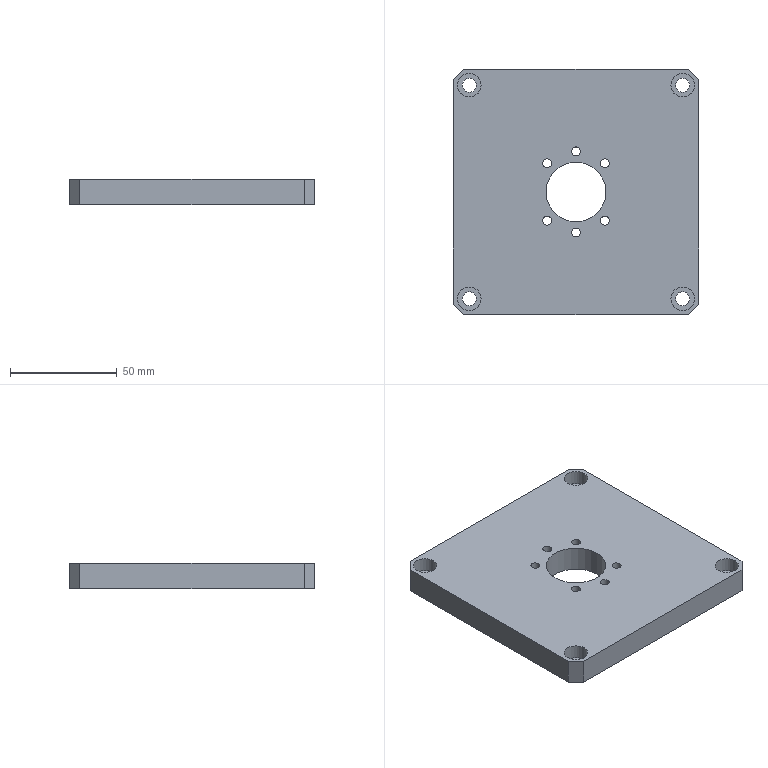Part | NX | 1 solid | 33 faces | box 115 x 115 x 12 mm | volume 146316 mm3 | cylinder 17 | plane 14 | cone 2 | commonest cylinder face diameters 4.2 x6 6.6 x4 11 x4 2.5 x2 28 x1
STEP:
#1=CARTESIAN_POINT('',(52.5,-57.5,6.));
#2=VERTEX_POINT('',#1);
#3=CARTESIAN_POINT('',(57.5,-52.5,6.));
#4=VERTEX_POINT('',#3);
#5=CARTESIAN_POINT('',(55.,-55.,6.));
#6=DIRECTION('',(0.7071,0.7071,0.));
#7=VECTOR('',#6,1000.);
#8=LINE('',#5,#7);
#9=EDGE_CURVE('',#2,#4,#8,.T.);
#10=ORIENTED_EDGE('',*,*,#9,.F.);
#11=CARTESIAN_POINT('',(52.5,-57.5,-6.));
#12=VERTEX_POINT('',#11);
#13=CARTESIAN_POINT('',(52.5,-57.5,6.));
#14=DIRECTION('',(0.,0.,1.));
#15=VECTOR('',#14,1000.);
#16=LINE('',#13,#15);
#17=EDGE_CURVE('',#12,#2,#16,.T.);
#18=ORIENTED_EDGE('',*,*,#17,.F.);
#19=CARTESIAN_POINT('',(57.5,-52.5,-6.));
#20=VERTEX_POINT('',#19);
#21=CARTESIAN_POINT('',(57.5,-52.5,-6.));
#22=DIRECTION('',(-0.7071,-0.7071,0.));
#23=VECTOR('',#22,1000.);
#24=LINE('',#21,#23);
#25=EDGE_CURVE('',#20,#12,#24,.T.);
#26=ORIENTED_EDGE('',*,*,#25,.F.);
#27=CARTESIAN_POINT('',(57.5,-52.5,6.));
#28=DIRECTION('',(0.,0.,-1.));
#29=VECTOR('',#28,1000.);
#30=LINE('',#27,#29);
#31=EDGE_CURVE('',#4,#20,#30,.T.);
#32=ORIENTED_EDGE('',*,*,#31,.F.);
#33=EDGE_LOOP('',(#10,#18,#26,#32));
#34=FACE_BOUND('',#33,.T.);
#35=CARTESIAN_POINT('',(57.5,-52.5,6.));
#36=DIRECTION('',(-0.7071,0.7071,0.));
#37=DIRECTION('',(0.,0.,-1.));
#38=AXIS2_PLACEMENT_3D('',#35,#36,#37);
#39=PLANE('',#38);
#40=ADVANCED_FACE('',(#34),#39,.F.);
#41=CARTESIAN_POINT('',(-57.5,-52.5,6.));
#42=VERTEX_POINT('',#41);
#43=CARTESIAN_POINT('',(-52.5,-57.5,6.));
#44=VERTEX_POINT('',#43);
#45=CARTESIAN_POINT('',(-55.,-55.,6.));
#46=DIRECTION('',(0.7071,-0.7071,0.));
#47=VECTOR('',#46,1000.);
#48=LINE('',#45,#47);
#49=EDGE_CURVE('',#42,#44,#48,.T.);
#50=ORIENTED_EDGE('',*,*,#49,.F.);
#51=CARTESIAN_POINT('',(-57.5,-52.5,-6.));
#52=VERTEX_POINT('',#51);
#53=CARTESIAN_POINT('',(-57.5,-52.5,6.));
#54=DIRECTION('',(0.,0.,1.));
#55=VECTOR('',#54,1000.);
#56=LINE('',#53,#55);
#57=EDGE_CURVE('',#52,#42,#56,.T.);
#58=ORIENTED_EDGE('',*,*,#57,.F.);
#59=CARTESIAN_POINT('',(-52.5,-57.5,-6.));
#60=VERTEX_POINT('',#59);
#61=CARTESIAN_POINT('',(-52.5,-57.5,-6.));
#62=DIRECTION('',(-0.7071,0.7071,0.));
#63=VECTOR('',#62,1000.);
#64=LINE('',#61,#63);
#65=EDGE_CURVE('',#60,#52,#64,.T.);
#66=ORIENTED_EDGE('',*,*,#65,.F.);
#67=CARTESIAN_POINT('',(-52.5,-57.5,6.));
#68=DIRECTION('',(0.,0.,-1.));
#69=VECTOR('',#68,1000.);
#70=LINE('',#67,#69);
#71=EDGE_CURVE('',#44,#60,#70,.T.);
#72=ORIENTED_EDGE('',*,*,#71,.F.);
#73=EDGE_LOOP('',(#50,#58,#66,#72));
#74=FACE_BOUND('',#73,.T.);
#75=CARTESIAN_POINT('',(-52.5,-57.5,6.));
#76=DIRECTION('',(0.7071,0.7071,0.));
#77=DIRECTION('',(0.,0.,-1.));
#78=AXIS2_PLACEMENT_3D('',#75,#76,#77);
#79=PLANE('',#78);
#80=ADVANCED_FACE('',(#74),#79,.F.);
#81=CARTESIAN_POINT('',(57.5,52.5,6.));
#82=VERTEX_POINT('',#81);
#83=CARTESIAN_POINT('',(52.5,57.5,6.));
#84=VERTEX_POINT('',#83);
#85=CARTESIAN_POINT('',(55.,55.,6.));
#86=DIRECTION('',(-0.7071,0.7071,0.));
#87=VECTOR('',#86,1000.);
#88=LINE('',#85,#87);
#89=EDGE_CURVE('',#82,#84,#88,.T.);
#90=ORIENTED_EDGE('',*,*,#89,.F.);
#91=CARTESIAN_POINT('',(57.5,52.5,-6.));
#92=VERTEX_POINT('',#91);
#93=CARTESIAN_POINT('',(57.5,52.5,6.));
#94=DIRECTION('',(0.,0.,1.));
#95=VECTOR('',#94,1000.);
#96=LINE('',#93,#95);
#97=EDGE_CURVE('',#92,#82,#96,.T.);
#98=ORIENTED_EDGE('',*,*,#97,.F.);
#99=CARTESIAN_POINT('',(52.5,57.5,-6.));
#100=VERTEX_POINT('',#99);
#101=CARTESIAN_POINT('',(52.5,57.5,-6.));
#102=DIRECTION('',(0.7071,-0.7071,0.));
#103=VECTOR('',#102,1000.);
#104=LINE('',#101,#103);
#105=EDGE_CURVE('',#100,#92,#104,.T.);
#106=ORIENTED_EDGE('',*,*,#105,.F.);
#107=CARTESIAN_POINT('',(52.5,57.5,6.));
#108=DIRECTION('',(0.,0.,-1.));
#109=VECTOR('',#108,1000.);
#110=LINE('',#107,#109);
#111=EDGE_CURVE('',#84,#100,#110,.T.);
#112=ORIENTED_EDGE('',*,*,#111,.F.);
#113=EDGE_LOOP('',(#90,#98,#106,#112));
#114=FACE_BOUND('',#113,.T.);
#115=CARTESIAN_POINT('',(52.5,57.5,6.));
#116=DIRECTION('',(-0.7071,-0.7071,0.));
#117=DIRECTION('',(0.,0.,-1.));
#118=AXIS2_PLACEMENT_3D('',#115,#116,#117);
#119=PLANE('',#118);
#120=ADVANCED_FACE('',(#114),#119,.F.);
#121=CARTESIAN_POINT('',(-52.5,57.5,6.));
#122=VERTEX_POINT('',#121);
#123=CARTESIAN_POINT('',(-57.5,52.5,6.));
#124=VERTEX_POINT('',#123);
#125=CARTESIAN_POINT('',(-55.,55.,6.));
#126=DIRECTION('',(-0.7071,-0.7071,0.));
#127=VECTOR('',#126,1000.);
#128=LINE('',#125,#127);
#129=EDGE_CURVE('',#122,#124,#128,.T.);
#130=ORIENTED_EDGE('',*,*,#129,.F.);
#131=CARTESIAN_POINT('',(-52.5,57.5,-6.));
#132=VERTEX_POINT('',#131);
#133=CARTESIAN_POINT('',(-52.5,57.5,6.));
#134=DIRECTION('',(0.,0.,1.));
#135=VECTOR('',#134,1000.);
#136=LINE('',#133,#135);
#137=EDGE_CURVE('',#132,#122,#136,.T.);
#138=ORIENTED_EDGE('',*,*,#137,.F.);
#139=CARTESIAN_POINT('',(-57.5,52.5,-6.));
#140=VERTEX_POINT('',#139);
#141=CARTESIAN_POINT('',(-57.5,52.5,-6.));
#142=DIRECTION('',(0.7071,0.7071,0.));
#143=VECTOR('',#142,1000.);
#144=LINE('',#141,#143);
#145=EDGE_CURVE('',#140,#132,#144,.T.);
#146=ORIENTED_EDGE('',*,*,#145,.F.);
#147=CARTESIAN_POINT('',(-57.5,52.5,6.));
#148=DIRECTION('',(0.,0.,-1.));
#149=VECTOR('',#148,1000.);
#150=LINE('',#147,#149);
#151=EDGE_CURVE('',#124,#140,#150,.T.);
#152=ORIENTED_EDGE('',*,*,#151,.F.);
#153=EDGE_LOOP('',(#130,#138,#146,#152));
#154=FACE_BOUND('',#153,.T.);
#155=CARTESIAN_POINT('',(-57.5,52.5,6.));
#156=DIRECTION('',(0.7071,-0.7071,0.));
#157=DIRECTION('',(0.,0.,-1.));
#158=AXIS2_PLACEMENT_3D('',#155,#156,#157);
#159=PLANE('',#158);
#160=ADVANCED_FACE('',(#154),#159,.F.);
#161=CARTESIAN_POINT('',(55.5,50.,-0.8));
#162=VERTEX_POINT('',#161);
#163=CARTESIAN_POINT('',(50.,50.,-0.8));
#164=DIRECTION('',(0.,0.,1.));
#165=DIRECTION('',(1.,0.,0.));
#166=AXIS2_PLACEMENT_3D('',#163,#164,#165);
#167=CIRCLE('',#166,5.5);
#168=EDGE_CURVE('',#162,#162,#167,.T.);
#169=ORIENTED_EDGE('',*,*,#168,.T.);
#170=EDGE_LOOP('',(#169));
#171=FACE_BOUND('',#170,.T.);
#172=CARTESIAN_POINT('',(53.3,50.,-0.8));
#173=VERTEX_POINT('',#172);
#174=CARTESIAN_POINT('',(50.,50.,-0.8));
#175=DIRECTION('',(0.,0.,1.));
#176=DIRECTION('',(1.,0.,0.));
#177=AXIS2_PLACEMENT_3D('',#174,#175,#176);
#178=CIRCLE('',#177,3.3);
#179=EDGE_CURVE('',#173,#173,#178,.T.);
#180=ORIENTED_EDGE('',*,*,#179,.F.);
#181=EDGE_LOOP('',(#180));
#182=FACE_BOUND('',#181,.T.);
#183=CARTESIAN_POINT('',(53.3,50.,-0.8));
#184=DIRECTION('',(0.,0.,-1.));
#185=DIRECTION('',(-1.,0.,0.));
#186=AXIS2_PLACEMENT_3D('',#183,#184,#185);
#187=PLANE('',#186);
#188=ADVANCED_FACE('',(#171,#182),#187,.F.);
#189=CARTESIAN_POINT('',(-55.5,50.,-0.8));
#190=VERTEX_POINT('',#189);
#191=CARTESIAN_POINT('',(-50.,50.,-0.8));
#192=DIRECTION('',(0.,0.,1.));
#193=DIRECTION('',(-1.,0.,0.));
#194=AXIS2_PLACEMENT_3D('',#191,#192,#193);
#195=CIRCLE('',#194,5.5);
#196=EDGE_CURVE('',#190,#190,#195,.T.);
#197=ORIENTED_EDGE('',*,*,#196,.T.);
#198=EDGE_LOOP('',(#197));
#199=FACE_BOUND('',#198,.T.);
#200=CARTESIAN_POINT('',(-53.3,50.,-0.8));
#201=VERTEX_POINT('',#200);
#202=CARTESIAN_POINT('',(-50.,50.,-0.8));
#203=DIRECTION('',(0.,0.,1.));
#204=DIRECTION('',(-1.,0.,0.));
#205=AXIS2_PLACEMENT_3D('',#202,#203,#204);
#206=CIRCLE('',#205,3.3);
#207=EDGE_CURVE('',#201,#201,#206,.T.);
#208=ORIENTED_EDGE('',*,*,#207,.F.);
#209=EDGE_LOOP('',(#208));
#210=FACE_BOUND('',#209,.T.);
#211=CARTESIAN_POINT('',(53.3,50.,-0.8));
#212=DIRECTION('',(0.,0.,-1.));
#213=DIRECTION('',(-1.,0.,0.));
#214=AXIS2_PLACEMENT_3D('',#211,#212,#213);
#215=PLANE('',#214);
#216=ADVANCED_FACE('',(#199,#210),#215,.F.);
#217=CARTESIAN_POINT('',(53.3,-50.,-6.));
#218=VERTEX_POINT('',#217);
#219=CARTESIAN_POINT('',(50.,-50.,-6.));
#220=DIRECTION('',(0.,0.,1.));
#221=DIRECTION('',(1.,0.,0.));
#222=AXIS2_PLACEMENT_3D('',#219,#220,#221);
#223=CIRCLE('',#222,3.3);
#224=EDGE_CURVE('',#218,#218,#223,.T.);
#225=ORIENTED_EDGE('',*,*,#224,.T.);
#226=EDGE_LOOP('',(#225));
#227=FACE_BOUND('',#226,.T.);
#228=CARTESIAN_POINT('',(-46.7,-50.,-6.));
#229=VERTEX_POINT('',#228);
#230=CARTESIAN_POINT('',(-50.,-50.,-6.));
#231=DIRECTION('',(0.,0.,1.));
#232=DIRECTION('',(1.,0.,0.));
#233=AXIS2_PLACEMENT_3D('',#230,#231,#232);
#234=CIRCLE('',#233,3.3);
#235=EDGE_CURVE('',#229,#229,#234,.T.);
#236=ORIENTED_EDGE('',*,*,#235,.T.);
#237=EDGE_LOOP('',(#236));
#238=FACE_BOUND('',#237,.T.);
#239=CARTESIAN_POINT('',(-57.5,57.5,-6.));
#240=DIRECTION('',(0.,-1.,0.));
#241=VECTOR('',#240,1000.);
#242=LINE('',#239,#241);
#243=EDGE_CURVE('',#140,#52,#242,.T.);
#244=ORIENTED_EDGE('',*,*,#243,.F.);
#245=ORIENTED_EDGE('',*,*,#145,.T.);
#246=CARTESIAN_POINT('',(-57.5,57.5,-6.));
#247=DIRECTION('',(-1.,0.,0.));
#248=VECTOR('',#247,1000.);
#249=LINE('',#246,#248);
#250=EDGE_CURVE('',#100,#132,#249,.T.);
#251=ORIENTED_EDGE('',*,*,#250,.F.);
#252=ORIENTED_EDGE('',*,*,#105,.T.);
#253=CARTESIAN_POINT('',(57.5,57.5,-6.));
#254=DIRECTION('',(0.,1.,0.));
#255=VECTOR('',#254,1000.);
#256=LINE('',#253,#255);
#257=EDGE_CURVE('',#20,#92,#256,.T.);
#258=ORIENTED_EDGE('',*,*,#257,.F.);
#259=ORIENTED_EDGE('',*,*,#25,.T.);
#260=CARTESIAN_POINT('',(-57.5,-57.5,-6.));
#261=DIRECTION('',(1.,0.,0.));
#262=VECTOR('',#261,1000.);
#263=LINE('',#260,#262);
#264=EDGE_CURVE('',#60,#12,#263,.T.);
#265=ORIENTED_EDGE('',*,*,#264,.F.);
#266=ORIENTED_EDGE('',*,*,#65,.T.);
#267=EDGE_LOOP('',(#244,#245,#251,#252,#258,#259,#265,#266));
#268=FACE_BOUND('',#267,.T.);
#269=CARTESIAN_POINT('',(-46.7,50.,-6.));
#270=VERTEX_POINT('',#269);
#271=CARTESIAN_POINT('',(-50.,50.,-6.));
#272=DIRECTION('',(0.,0.,1.));
#273=DIRECTION('',(1.,0.,0.));
#274=AXIS2_PLACEMENT_3D('',#271,#272,#273);
#275=CIRCLE('',#274,3.3);
#276=EDGE_CURVE('',#270,#270,#275,.T.);
#277=ORIENTED_EDGE('',*,*,#276,.T.);
#278=EDGE_LOOP('',(#277));
#279=FACE_BOUND('',#278,.T.);
#280=CARTESIAN_POINT('',(53.3,50.,-6.));
#281=VERTEX_POINT('',#280);
#282=CARTESIAN_POINT('',(50.,50.,-6.));
#283=DIRECTION('',(0.,0.,1.));
#284=DIRECTION('',(1.,0.,0.));
#285=AXIS2_PLACEMENT_3D('',#282,#283,#284);
#286=CIRCLE('',#285,3.3);
#287=EDGE_CURVE('',#281,#281,#286,.T.);
#288=ORIENTED_EDGE('',*,*,#287,.T.);
#289=EDGE_LOOP('',(#288));
#290=FACE_BOUND('',#289,.T.);
#291=CARTESIAN_POINT('',(-14.,0.,-6.));
#292=VERTEX_POINT('',#291);
#293=CARTESIAN_POINT('',(0.,0.,-6.));
#294=DIRECTION('',(0.,0.,-1.));
#295=DIRECTION('',(-1.,0.,0.));
#296=AXIS2_PLACEMENT_3D('',#293,#294,#295);
#297=CIRCLE('',#296,14.);
#298=EDGE_CURVE('',#292,#292,#297,.T.);
#299=ORIENTED_EDGE('',*,*,#298,.F.);
#300=EDGE_LOOP('',(#299));
#301=FACE_BOUND('',#300,.T.);
#302=CARTESIAN_POINT('',(15.535,-13.435,-6.));
#303=VERTEX_POINT('',#302);
#304=CARTESIAN_POINT('',(13.435,-13.435,-6.));
#305=DIRECTION('',(0.,0.,1.));
#306=DIRECTION('',(1.,0.,0.));
#307=AXIS2_PLACEMENT_3D('',#304,#305,#306);
#308=CIRCLE('',#307,2.1);
#309=EDGE_CURVE('',#303,#303,#308,.T.);
#310=ORIENTED_EDGE('',*,*,#309,.T.);
#311=EDGE_LOOP('',(#310));
#312=FACE_BOUND('',#311,.T.);
#313=CARTESIAN_POINT('',(2.1,-19.,-6.));
#314=VERTEX_POINT('',#313);
#315=CARTESIAN_POINT('',(0.,-19.,-6.));
#316=DIRECTION('',(0.,0.,1.));
#317=DIRECTION('',(1.,0.,0.));
#318=AXIS2_PLACEMENT_3D('',#315,#316,#317);
#319=CIRCLE('',#318,2.1);
#320=EDGE_CURVE('',#314,#314,#319,.T.);
#321=ORIENTED_EDGE('',*,*,#320,.T.);
#322=EDGE_LOOP('',(#321));
#323=FACE_BOUND('',#322,.T.);
#324=CARTESIAN_POINT('',(-11.335,-13.435,-6.));
#325=VERTEX_POINT('',#324);
#326=CARTESIAN_POINT('',(-13.435,-13.435,-6.));
#327=DIRECTION('',(0.,0.,1.));
#328=DIRECTION('',(1.,0.,0.));
#329=AXIS2_PLACEMENT_3D('',#326,#327,#328);
#330=CIRCLE('',#329,2.1);
#331=EDGE_CURVE('',#325,#325,#330,.T.);
#332=ORIENTED_EDGE('',*,*,#331,.T.);
#333=EDGE_LOOP('',(#332));
#334=FACE_BOUND('',#333,.T.);
#335=CARTESIAN_POINT('',(15.535,13.435,-6.));
#336=VERTEX_POINT('',#335);
#337=CARTESIAN_POINT('',(13.435,13.435,-6.));
#338=DIRECTION('',(0.,0.,1.));
#339=DIRECTION('',(1.,0.,0.));
#340=AXIS2_PLACEMENT_3D('',#337,#338,#339);
#341=CIRCLE('',#340,2.1);
#342=EDGE_CURVE('',#336,#336,#341,.T.);
#343=ORIENTED_EDGE('',*,*,#342,.T.);
#344=EDGE_LOOP('',(#343));
#345=FACE_BOUND('',#344,.T.);
#346=CARTESIAN_POINT('',(-11.335,13.435,-6.));
#347=VERTEX_POINT('',#346);
#348=CARTESIAN_POINT('',(-13.435,13.435,-6.));
#349=DIRECTION('',(0.,0.,1.));
#350=DIRECTION('',(1.,0.,0.));
#351=AXIS2_PLACEMENT_3D('',#348,#349,#350);
#352=CIRCLE('',#351,2.1);
#353=EDGE_CURVE('',#347,#347,#352,.T.);
#354=ORIENTED_EDGE('',*,*,#353,.T.);
#355=EDGE_LOOP('',(#354));
#356=FACE_BOUND('',#355,.T.);
#357=CARTESIAN_POINT('',(2.1,19.,-6.));
#358=VERTEX_POINT('',#357);
#359=CARTESIAN_POINT('',(0.,19.,-6.));
#360=DIRECTION('',(0.,0.,1.));
#361=DIRECTION('',(1.,0.,0.));
#362=AXIS2_PLACEMENT_3D('',#359,#360,#361);
#363=CIRCLE('',#362,2.1);
#364=EDGE_CURVE('',#358,#358,#363,.T.);
#365=ORIENTED_EDGE('',*,*,#364,.T.);
#366=EDGE_LOOP('',(#365));
#367=FACE_BOUND('',#366,.T.);
#368=CARTESIAN_POINT('',(0.,0.,-6.));
#369=DIRECTION('',(0.,0.,1.));
#370=DIRECTION('',(1.,0.,0.));
#371=AXIS2_PLACEMENT_3D('',#368,#369,#370);
#372=PLANE('',#371);
#373=ADVANCED_FACE('',(#227,#238,#268,#279,#290,#301,#312,#323,#334,#345,#356,#367),#372,.F.);
#374=CARTESIAN_POINT('',(55.5,-50.,6.));
#375=VERTEX_POINT('',#374);
#376=CARTESIAN_POINT('',(50.,-50.,6.));
#377=DIRECTION('',(0.,0.,1.));
#378=DIRECTION('',(1.,0.,0.));
#379=AXIS2_PLACEMENT_3D('',#376,#377,#378);
#380=CIRCLE('',#379,5.5);
#381=EDGE_CURVE('',#375,#375,#380,.T.);
#382=ORIENTED_EDGE('',*,*,#381,.F.);
#383=EDGE_LOOP('',(#382));
#384=FACE_BOUND('',#383,.T.);
#385=CARTESIAN_POINT('',(-44.5,-50.,6.));
#386=VERTEX_POINT('',#385);
#387=CARTESIAN_POINT('',(-50.,-50.,6.));
#388=DIRECTION('',(0.,0.,1.));
#389=DIRECTION('',(1.,0.,0.));
#390=AXIS2_PLACEMENT_3D('',#387,#388,#389);
#391=CIRCLE('',#390,5.5);
#392=EDGE_CURVE('',#386,#386,#391,.T.);
#393=ORIENTED_EDGE('',*,*,#392,.F.);
#394=EDGE_LOOP('',(#393));
#395=FACE_BOUND('',#394,.T.);
#396=CARTESIAN_POINT('',(-57.5,57.5,6.));
#397=DIRECTION('',(-1.,0.,0.));
#398=VECTOR('',#397,1000.);
#399=LINE('',#396,#398);
#400=EDGE_CURVE('',#84,#122,#399,.T.);
#401=ORIENTED_EDGE('',*,*,#400,.T.);
#402=ORIENTED_EDGE('',*,*,#129,.T.);
#403=CARTESIAN_POINT('',(-57.5,57.5,6.));
#404=DIRECTION('',(0.,-1.,0.));
#405=VECTOR('',#404,1000.);
#406=LINE('',#403,#405);
#407=EDGE_CURVE('',#124,#42,#406,.T.);
#408=ORIENTED_EDGE('',*,*,#407,.T.);
#409=ORIENTED_EDGE('',*,*,#49,.T.);
#410=CARTESIAN_POINT('',(-57.5,-57.5,6.));
#411=DIRECTION('',(1.,0.,0.));
#412=VECTOR('',#411,1000.);
#413=LINE('',#410,#412);
#414=EDGE_CURVE('',#44,#2,#413,.T.);
#415=ORIENTED_EDGE('',*,*,#414,.T.);
#416=ORIENTED_EDGE('',*,*,#9,.T.);
#417=CARTESIAN_POINT('',(57.5,57.5,6.));
#418=DIRECTION('',(0.,1.,0.));
#419=VECTOR('',#418,1000.);
#420=LINE('',#417,#419);
#421=EDGE_CURVE('',#4,#82,#420,.T.);
#422=ORIENTED_EDGE('',*,*,#421,.T.);
#423=ORIENTED_EDGE('',*,*,#89,.T.);
#424=EDGE_LOOP('',(#401,#402,#408,#409,#415,#416,#422,#423));
#425=FACE_BOUND('',#424,.T.);
#426=CARTESIAN_POINT('',(-44.5,50.,6.));
#427=VERTEX_POINT('',#426);
#428=CARTESIAN_POINT('',(-50.,50.,6.));
#429=DIRECTION('',(0.,0.,1.));
#430=DIRECTION('',(1.,0.,0.));
#431=AXIS2_PLACEMENT_3D('',#428,#429,#430);
#432=CIRCLE('',#431,5.5);
#433=EDGE_CURVE('',#427,#427,#432,.T.);
#434=ORIENTED_EDGE('',*,*,#433,.F.);
#435=EDGE_LOOP('',(#434));
#436=FACE_BOUND('',#435,.T.);
#437=CARTESIAN_POINT('',(55.5,50.,6.));
#438=VERTEX_POINT('',#437);
#439=CARTESIAN_POINT('',(50.,50.,6.));
#440=DIRECTION('',(0.,0.,1.));
#441=DIRECTION('',(1.,0.,0.));
#442=AXIS2_PLACEMENT_3D('',#439,#440,#441);
#443=CIRCLE('',#442,5.5);
#444=EDGE_CURVE('',#438,#438,#443,.T.);
#445=ORIENTED_EDGE('',*,*,#444,.F.);
#446=EDGE_LOOP('',(#445));
#447=FACE_BOUND('',#446,.T.);
#448=CARTESIAN_POINT('',(14.,0.,6.));
#449=VERTEX_POINT('',#448);
#450=CARTESIAN_POINT('',(0.,0.,6.));
#451=DIRECTION('',(0.,0.,1.));
#452=DIRECTION('',(1.,0.,0.));
#453=AXIS2_PLACEMENT_3D('',#450,#451,#452);
#454=CIRCLE('',#453,14.);
#455=EDGE_CURVE('',#449,#449,#454,.T.);
#456=ORIENTED_EDGE('',*,*,#455,.F.);
#457=EDGE_LOOP('',(#456));
#458=FACE_BOUND('',#457,.T.);
#459=CARTESIAN_POINT('',(15.535,-13.435,6.));
#460=VERTEX_POINT('',#459);
#461=CARTESIAN_POINT('',(13.435,-13.435,6.));
#462=DIRECTION('',(0.,0.,1.));
#463=DIRECTION('',(1.,0.,0.));
#464=AXIS2_PLACEMENT_3D('',#461,#462,#463);
#465=CIRCLE('',#464,2.1);
#466=EDGE_CURVE('',#460,#460,#465,.T.);
#467=ORIENTED_EDGE('',*,*,#466,.F.);
#468=EDGE_LOOP('',(#467));
#469=FACE_BOUND('',#468,.T.);
#470=CARTESIAN_POINT('',(2.1,-19.,6.));
#471=VERTEX_POINT('',#470);
#472=CARTESIAN_POINT('',(0.,-19.,6.));
#473=DIRECTION('',(0.,0.,1.));
#474=DIRECTION('',(1.,0.,0.));
#475=AXIS2_PLACEMENT_3D('',#472,#473,#474);
#476=CIRCLE('',#475,2.1);
#477=EDGE_CURVE('',#471,#471,#476,.T.);
#478=ORIENTED_EDGE('',*,*,#477,.F.);
#479=EDGE_LOOP('',(#478));
#480=FACE_BOUND('',#479,.T.);
#481=CARTESIAN_POINT('',(-11.335,-13.435,6.));
#482=VERTEX_POINT('',#481);
#483=CARTESIAN_POINT('',(-13.435,-13.435,6.));
#484=DIRECTION('',(0.,0.,1.));
#485=DIRECTION('',(1.,0.,0.));
#486=AXIS2_PLACEMENT_3D('',#483,#484,#485);
#487=CIRCLE('',#486,2.1);
#488=EDGE_CURVE('',#482,#482,#487,.T.);
#489=ORIENTED_EDGE('',*,*,#488,.F.);
#490=EDGE_LOOP('',(#489));
#491=FACE_BOUND('',#490,.T.);
#492=CARTESIAN_POINT('',(15.535,13.435,6.));
#493=VERTEX_POINT('',#492);
#494=CARTESIAN_POINT('',(13.435,13.435,6.));
#495=DIRECTION('',(0.,0.,1.));
#496=DIRECTION('',(1.,0.,0.));
#497=AXIS2_PLACEMENT_3D('',#494,#495,#496);
#498=CIRCLE('',#497,2.1);
#499=EDGE_CURVE('',#493,#493,#498,.T.);
#500=ORIENTED_EDGE('',*,*,#499,.F.);
#501=EDGE_LOOP('',(#500));
#502=FACE_BOUND('',#501,.T.);
#503=CARTESIAN_POINT('',(-11.335,13.435,6.));
#504=VERTEX_POINT('',#503);
#505=CARTESIAN_POINT('',(-13.435,13.435,6.));
#506=DIRECTION('',(0.,0.,1.));
#507=DIRECTION('',(1.,0.,0.));
#508=AXIS2_PLACEMENT_3D('',#505,#506,#507);
#509=CIRCLE('',#508,2.1);
#510=EDGE_CURVE('',#504,#504,#509,.T.);
#511=ORIENTED_EDGE('',*,*,#510,.F.);
#512=EDGE_LOOP('',(#511));
#513=FACE_BOUND('',#512,.T.);
#514=CARTESIAN_POINT('',(2.1,19.,6.));
#515=VERTEX_POINT('',#514);
#516=CARTESIAN_POINT('',(0.,19.,6.));
#517=DIRECTION('',(0.,0.,1.));
#518=DIRECTION('',(1.,0.,0.));
#519=AXIS2_PLACEMENT_3D('',#516,#517,#518);
#520=CIRCLE('',#519,2.1);
#521=EDGE_CURVE('',#515,#515,#520,.T.);
#522=ORIENTED_EDGE('',*,*,#521,.F.);
#523=EDGE_LOOP('',(#522));
#524=FACE_BOUND('',#523,.T.);
#525=CARTESIAN_POINT('',(0.,0.,6.));
#526=DIRECTION('',(0.,0.,1.));
#527=DIRECTION('',(1.,0.,0.));
#528=AXIS2_PLACEMENT_3D('',#525,#526,#527);
#529=PLANE('',#528);
#530=ADVANCED_FACE('',(#384,#395,#425,#436,#447,#458,#469,#480,#491,#502,#513,#524),#529,.T.);
#531=ORIENTED_EDGE('',*,*,#414,.F.);
#532=ORIENTED_EDGE('',*,*,#71,.T.);
#533=ORIENTED_EDGE('',*,*,#264,.T.);
#534=ORIENTED_EDGE('',*,*,#17,.T.);
#535=EDGE_LOOP('',(#531,#532,#533,#534));
#536=FACE_BOUND('',#535,.T.);
#537=CARTESIAN_POINT('',(-57.5,-57.5,6.));
#538=DIRECTION('',(0.,1.,0.));
#539=DIRECTION('',(0.,0.,1.));
#540=AXIS2_PLACEMENT_3D('',#537,#538,#539);
#541=PLANE('',#540);
#542=ADVANCED_FACE('',(#536),#541,.F.);
#543=ORIENTED_EDGE('',*,*,#407,.F.);
#544=ORIENTED_EDGE('',*,*,#151,.T.);
#545=ORIENTED_EDGE('',*,*,#243,.T.);
#546=ORIENTED_EDGE('',*,*,#57,.T.);
#547=EDGE_LOOP('',(#543,#544,#545,#546));
#548=FACE_BOUND('',#547,.T.);
#549=CARTESIAN_POINT('',(-57.5,57.5,6.));
#550=DIRECTION('',(1.,0.,0.));
#551=DIRECTION('',(0.,1.,0.));
#552=AXIS2_PLACEMENT_3D('',#549,#550,#551);
#553=PLANE('',#552);
#554=ADVANCED_FACE('',(#548),#553,.F.);
#555=ORIENTED_EDGE('',*,*,#250,.T.);
#556=ORIENTED_EDGE('',*,*,#137,.T.);
#557=ORIENTED_EDGE('',*,*,#400,.F.);
#558=ORIENTED_EDGE('',*,*,#111,.T.);
#559=EDGE_LOOP('',(#555,#556,#557,#558));
#560=FACE_BOUND('',#559,.T.);
#561=CARTESIAN_POINT('',(32.5,57.5,1.25));
#562=VERTEX_POINT('',#561);
#563=CARTESIAN_POINT('',(32.5,57.5,0.));
#564=DIRECTION('',(0.,1.,0.));
#565=DIRECTION('',(0.,0.,1.));
#566=AXIS2_PLACEMENT_3D('',#563,#564,#565);
#567=CIRCLE('',#566,1.25);
#568=EDGE_CURVE('',#562,#562,#567,.T.);
#569=ORIENTED_EDGE('',*,*,#568,.F.);
#570=EDGE_LOOP('',(#569));
#571=FACE_BOUND('',#570,.T.);
#572=CARTESIAN_POINT('',(22.5,57.5,1.25));
#573=VERTEX_POINT('',#572);
#574=CARTESIAN_POINT('',(22.5,57.5,0.));
#575=DIRECTION('',(0.,1.,0.));
#576=DIRECTION('',(0.,0.,1.));
#577=AXIS2_PLACEMENT_3D('',#574,#575,#576);
#578=CIRCLE('',#577,1.25);
#579=EDGE_CURVE('',#573,#573,#578,.T.);
#580=ORIENTED_EDGE('',*,*,#579,.F.);
#581=EDGE_LOOP('',(#580));
#582=FACE_BOUND('',#581,.T.);
#583=CARTESIAN_POINT('',(-57.5,57.5,6.));
#584=DIRECTION('',(0.,-1.,0.));
#585=DIRECTION('',(0.,0.,-1.));
#586=AXIS2_PLACEMENT_3D('',#583,#584,#585);
#587=PLANE('',#586);
#588=ADVANCED_FACE('',(#560,#571,#582),#587,.F.);
#589=ORIENTED_EDGE('',*,*,#257,.T.);
#590=ORIENTED_EDGE('',*,*,#97,.T.);
#591=ORIENTED_EDGE('',*,*,#421,.F.);
#592=ORIENTED_EDGE('',*,*,#31,.T.);
#593=EDGE_LOOP('',(#589,#590,#591,#592));
#594=FACE_BOUND('',#593,.T.);
#595=CARTESIAN_POINT('',(57.5,57.5,6.));
#596=DIRECTION('',(-1.,0.,0.));
#597=DIRECTION('',(0.,-1.,0.));
#598=AXIS2_PLACEMENT_3D('',#595,#596,#597);
#599=PLANE('',#598);
#600=ADVANCED_FACE('',(#594),#599,.F.);
#601=CARTESIAN_POINT('',(-55.5,-50.,-0.8));
#602=VERTEX_POINT('',#601);
#603=CARTESIAN_POINT('',(-50.,-50.,-0.8));
#604=DIRECTION('',(0.,0.,1.));
#605=DIRECTION('',(-1.,0.,0.));
#606=AXIS2_PLACEMENT_3D('',#603,#604,#605);
#607=CIRCLE('',#606,5.5);
#608=EDGE_CURVE('',#602,#602,#607,.T.);
#609=ORIENTED_EDGE('',*,*,#608,.T.);
#610=EDGE_LOOP('',(#609));
#611=FACE_BOUND('',#610,.T.);
#612=CARTESIAN_POINT('',(-53.3,-50.,-0.8));
#613=VERTEX_POINT('',#612);
#614=CARTESIAN_POINT('',(-50.,-50.,-0.8));
#615=DIRECTION('',(0.,0.,1.));
#616=DIRECTION('',(-1.,0.,0.));
#617=AXIS2_PLACEMENT_3D('',#614,#615,#616);
#618=CIRCLE('',#617,3.3);
#619=EDGE_CURVE('',#613,#613,#618,.T.);
#620=ORIENTED_EDGE('',*,*,#619,.F.);
#621=EDGE_LOOP('',(#620));
#622=FACE_BOUND('',#621,.T.);
#623=CARTESIAN_POINT('',(53.3,50.,-0.8));
#624=DIRECTION('',(0.,0.,-1.));
#625=DIRECTION('',(-1.,0.,0.));
#626=AXIS2_PLACEMENT_3D('',#623,#624,#625);
#627=PLANE('',#626);
#628=ADVANCED_FACE('',(#611,#622),#627,.F.);
#629=CARTESIAN_POINT('',(44.5,-50.,-0.8));
#630=VERTEX_POINT('',#629);
#631=CARTESIAN_POINT('',(50.,-50.,-0.8));
#632=DIRECTION('',(0.,0.,1.));
#633=DIRECTION('',(-1.,0.,0.));
#634=AXIS2_PLACEMENT_3D('',#631,#632,#633);
#635=CIRCLE('',#634,5.5);
#636=EDGE_CURVE('',#630,#630,#635,.T.);
#637=ORIENTED_EDGE('',*,*,#636,.T.);
#638=EDGE_LOOP('',(#637));
#639=FACE_BOUND('',#638,.T.);
#640=CARTESIAN_POINT('',(46.7,-50.,-0.8));
#641=VERTEX_POINT('',#640);
#642=CARTESIAN_POINT('',(50.,-50.,-0.8));
#643=DIRECTION('',(0.,0.,1.));
#644=DIRECTION('',(-1.,0.,0.));
#645=AXIS2_PLACEMENT_3D('',#642,#643,#644);
#646=CIRCLE('',#645,3.3);
#647=EDGE_CURVE('',#641,#641,#646,.T.);
#648=ORIENTED_EDGE('',*,*,#647,.F.);
#649=EDGE_LOOP('',(#648));
#650=FACE_BOUND('',#649,.T.);
#651=CARTESIAN_POINT('',(53.3,50.,-0.8));
#652=DIRECTION('',(0.,0.,-1.));
#653=DIRECTION('',(-1.,0.,0.));
#654=AXIS2_PLACEMENT_3D('',#651,#652,#653);
#655=PLANE('',#654);
#656=ADVANCED_FACE('',(#639,#650),#655,.F.);
#657=ORIENTED_EDGE('',*,*,#636,.F.);
#658=EDGE_LOOP('',(#657));
#659=FACE_BOUND('',#658,.T.);
#660=ORIENTED_EDGE('',*,*,#381,.T.);
#661=EDGE_LOOP('',(#660));
#662=FACE_BOUND('',#661,.T.);
#663=CARTESIAN_POINT('',(50.,-50.,6.));
#664=DIRECTION('',(0.,0.,1.));
#665=DIRECTION('',(1.,0.,0.));
#666=AXIS2_PLACEMENT_3D('',#663,#664,#665);
#667=CYLINDRICAL_SURFACE('',#666,5.5);
#668=ADVANCED_FACE('',(#659,#662),#667,.F.);
#669=ORIENTED_EDGE('',*,*,#224,.F.);
#670=EDGE_LOOP('',(#669));
#671=FACE_BOUND('',#670,.T.);
#672=ORIENTED_EDGE('',*,*,#647,.T.);
#673=EDGE_LOOP('',(#672));
#674=FACE_BOUND('',#673,.T.);
#675=CARTESIAN_POINT('',(50.,-50.,6.));
#676=DIRECTION('',(0.,0.,1.));
#677=DIRECTION('',(1.,0.,0.));
#678=AXIS2_PLACEMENT_3D('',#675,#676,#677);
#679=CYLINDRICAL_SURFACE('',#678,3.3);
#680=ADVANCED_FACE('',(#671,#674),#679,.F.);
#681=ORIENTED_EDGE('',*,*,#608,.F.);
#682=EDGE_LOOP('',(#681));
#683=FACE_BOUND('',#682,.T.);
#684=ORIENTED_EDGE('',*,*,#392,.T.);
#685=EDGE_LOOP('',(#684));
#686=FACE_BOUND('',#685,.T.);
#687=CARTESIAN_POINT('',(-50.,-50.,6.));
#688=DIRECTION('',(0.,0.,1.));
#689=DIRECTION('',(1.,0.,0.));
#690=AXIS2_PLACEMENT_3D('',#687,#688,#689);
#691=CYLINDRICAL_SURFACE('',#690,5.5);
#692=ADVANCED_FACE('',(#683,#686),#691,.F.);
#693=ORIENTED_EDGE('',*,*,#235,.F.);
#694=EDGE_LOOP('',(#693));
#695=FACE_BOUND('',#694,.T.);
#696=ORIENTED_EDGE('',*,*,#619,.T.);
#697=EDGE_LOOP('',(#696));
#698=FACE_BOUND('',#697,.T.);
#699=CARTESIAN_POINT('',(-50.,-50.,6.));
#700=DIRECTION('',(0.,0.,1.));
#701=DIRECTION('',(1.,0.,0.));
#702=AXIS2_PLACEMENT_3D('',#699,#700,#701);
#703=CYLINDRICAL_SURFACE('',#702,3.3);
#704=ADVANCED_FACE('',(#695,#698),#703,.F.);
#705=ORIENTED_EDGE('',*,*,#276,.F.);
#706=EDGE_LOOP('',(#705));
#707=FACE_BOUND('',#706,.T.);
#708=ORIENTED_EDGE('',*,*,#207,.T.);
#709=EDGE_LOOP('',(#708));
#710=FACE_BOUND('',#709,.T.);
#711=CARTESIAN_POINT('',(-50.,50.,6.));
#712=DIRECTION('',(0.,0.,1.));
#713=DIRECTION('',(1.,0.,0.));
#714=AXIS2_PLACEMENT_3D('',#711,#712,#713);
#715=CYLINDRICAL_SURFACE('',#714,3.3);
#716=ADVANCED_FACE('',(#707,#710),#715,.F.);
#717=ORIENTED_EDGE('',*,*,#196,.F.);
#718=EDGE_LOOP('',(#717));
#719=FACE_BOUND('',#718,.T.);
#720=ORIENTED_EDGE('',*,*,#433,.T.);
#721=EDGE_LOOP('',(#720));
#722=FACE_BOUND('',#721,.T.);
#723=CARTESIAN_POINT('',(-50.,50.,6.));
#724=DIRECTION('',(0.,0.,1.));
#725=DIRECTION('',(1.,0.,0.));
#726=AXIS2_PLACEMENT_3D('',#723,#724,#725);
#727=CYLINDRICAL_SURFACE('',#726,5.5);
#728=ADVANCED_FACE('',(#719,#722),#727,.F.);
#729=ORIENTED_EDGE('',*,*,#287,.F.);
#730=EDGE_LOOP('',(#729));
#731=FACE_BOUND('',#730,.T.);
#732=ORIENTED_EDGE('',*,*,#179,.T.);
#733=EDGE_LOOP('',(#732));
#734=FACE_BOUND('',#733,.T.);
#735=CARTESIAN_POINT('',(50.,50.,6.));
#736=DIRECTION('',(0.,0.,1.));
#737=DIRECTION('',(1.,0.,0.));
#738=AXIS2_PLACEMENT_3D('',#735,#736,#737);
#739=CYLINDRICAL_SURFACE('',#738,3.3);
#740=ADVANCED_FACE('',(#731,#734),#739,.F.);
#741=ORIENTED_EDGE('',*,*,#168,.F.);
#742=EDGE_LOOP('',(#741));
#743=FACE_BOUND('',#742,.T.);
#744=ORIENTED_EDGE('',*,*,#444,.T.);
#745=EDGE_LOOP('',(#744));
#746=FACE_BOUND('',#745,.T.);
#747=CARTESIAN_POINT('',(50.,50.,6.));
#748=DIRECTION('',(0.,0.,1.));
#749=DIRECTION('',(1.,0.,0.));
#750=AXIS2_PLACEMENT_3D('',#747,#748,#749);
#751=CYLINDRICAL_SURFACE('',#750,5.5);
#752=ADVANCED_FACE('',(#743,#746),#751,.F.);
#753=ORIENTED_EDGE('',*,*,#298,.T.);
#754=EDGE_LOOP('',(#753));
#755=FACE_BOUND('',#754,.T.);
#756=ORIENTED_EDGE('',*,*,#455,.T.);
#757=EDGE_LOOP('',(#756));
#758=FACE_BOUND('',#757,.T.);
#759=CARTESIAN_POINT('',(0.,0.,20.));
#760=DIRECTION('',(0.,0.,-1.));
#761=DIRECTION('',(-1.,0.,0.));
#762=AXIS2_PLACEMENT_3D('',#759,#760,#761);
#763=CYLINDRICAL_SURFACE('',#762,14.);
#764=ADVANCED_FACE('',(#755,#758),#763,.F.);
#765=ORIENTED_EDGE('',*,*,#309,.F.);
#766=EDGE_LOOP('',(#765));
#767=FACE_BOUND('',#766,.T.);
#768=ORIENTED_EDGE('',*,*,#466,.T.);
#769=EDGE_LOOP('',(#768));
#770=FACE_BOUND('',#769,.T.);
#771=CARTESIAN_POINT('',(13.435,-13.435,6.));
#772=DIRECTION('',(0.,0.,1.));
#773=DIRECTION('',(1.,0.,0.));
#774=AXIS2_PLACEMENT_3D('',#771,#772,#773);
#775=CYLINDRICAL_SURFACE('',#774,2.1);
#776=ADVANCED_FACE('',(#767,#770),#775,.F.);
#777=ORIENTED_EDGE('',*,*,#320,.F.);
#778=EDGE_LOOP('',(#777));
#779=FACE_BOUND('',#778,.T.);
#780=ORIENTED_EDGE('',*,*,#477,.T.);
#781=EDGE_LOOP('',(#780));
#782=FACE_BOUND('',#781,.T.);
#783=CARTESIAN_POINT('',(0.,-19.,6.));
#784=DIRECTION('',(0.,0.,1.));
#785=DIRECTION('',(1.,0.,0.));
#786=AXIS2_PLACEMENT_3D('',#783,#784,#785);
#787=CYLINDRICAL_SURFACE('',#786,2.1);
#788=ADVANCED_FACE('',(#779,#782),#787,.F.);
#789=ORIENTED_EDGE('',*,*,#331,.F.);
#790=EDGE_LOOP('',(#789));
#791=FACE_BOUND('',#790,.T.);
#792=ORIENTED_EDGE('',*,*,#488,.T.);
#793=EDGE_LOOP('',(#792));
#794=FACE_BOUND('',#793,.T.);
#795=CARTESIAN_POINT('',(-13.435,-13.435,6.));
#796=DIRECTION('',(0.,0.,1.));
#797=DIRECTION('',(1.,0.,0.));
#798=AXIS2_PLACEMENT_3D('',#795,#796,#797);
#799=CYLINDRICAL_SURFACE('',#798,2.1);
#800=ADVANCED_FACE('',(#791,#794),#799,.F.);
#801=ORIENTED_EDGE('',*,*,#342,.F.);
#802=EDGE_LOOP('',(#801));
#803=FACE_BOUND('',#802,.T.);
#804=ORIENTED_EDGE('',*,*,#499,.T.);
#805=EDGE_LOOP('',(#804));
#806=FACE_BOUND('',#805,.T.);
#807=CARTESIAN_POINT('',(13.435,13.435,6.));
#808=DIRECTION('',(0.,0.,1.));
#809=DIRECTION('',(1.,0.,0.));
#810=AXIS2_PLACEMENT_3D('',#807,#808,#809);
#811=CYLINDRICAL_SURFACE('',#810,2.1);
#812=ADVANCED_FACE('',(#803,#806),#811,.F.);
#813=ORIENTED_EDGE('',*,*,#353,.F.);
#814=EDGE_LOOP('',(#813));
#815=FACE_BOUND('',#814,.T.);
#816=ORIENTED_EDGE('',*,*,#510,.T.);
#817=EDGE_LOOP('',(#816));
#818=FACE_BOUND('',#817,.T.);
#819=CARTESIAN_POINT('',(-13.435,13.435,6.));
#820=DIRECTION('',(0.,0.,1.));
#821=DIRECTION('',(1.,0.,0.));
#822=AXIS2_PLACEMENT_3D('',#819,#820,#821);
#823=CYLINDRICAL_SURFACE('',#822,2.1);
#824=ADVANCED_FACE('',(#815,#818),#823,.F.);
#825=ORIENTED_EDGE('',*,*,#364,.F.);
#826=EDGE_LOOP('',(#825));
#827=FACE_BOUND('',#826,.T.);
#828=ORIENTED_EDGE('',*,*,#521,.T.);
#829=EDGE_LOOP('',(#828));
#830=FACE_BOUND('',#829,.T.);
#831=CARTESIAN_POINT('',(0.,19.,6.));
#832=DIRECTION('',(0.,0.,1.));
#833=DIRECTION('',(1.,0.,0.));
#834=AXIS2_PLACEMENT_3D('',#831,#832,#833);
#835=CYLINDRICAL_SURFACE('',#834,2.1);
#836=ADVANCED_FACE('',(#827,#830),#835,.F.);
#837=CARTESIAN_POINT('',(32.5,47.5,1.25));
#838=VERTEX_POINT('',#837);
#839=CARTESIAN_POINT('',(32.5,47.5,0.));
#840=DIRECTION('',(0.,1.,0.));
#841=DIRECTION('',(0.,0.,1.));
#842=AXIS2_PLACEMENT_3D('',#839,#840,#841);
#843=CIRCLE('',#842,1.25);
#844=EDGE_CURVE('',#838,#838,#843,.T.);
#845=ORIENTED_EDGE('',*,*,#844,.T.);
#846=EDGE_LOOP('',(#845));
#847=FACE_BOUND('',#846,.T.);
#848=CARTESIAN_POINT('',(32.5,46.749,0.));
#849=VERTEX_POINT('',#848);
#850=VERTEX_LOOP('',#849);
#851=FACE_BOUND('',#850,.T.);
#852=CARTESIAN_POINT('',(32.5,47.5,0.));
#853=DIRECTION('',(0.,1.,0.));
#854=DIRECTION('',(0.,0.,1.));
#855=AXIS2_PLACEMENT_3D('',#852,#853,#854);
#856=CONICAL_SURFACE('',#855,1.25,1.03);
#857=ADVANCED_FACE('',(#847,#851),#856,.F.);
#858=ORIENTED_EDGE('',*,*,#844,.F.);
#859=EDGE_LOOP('',(#858));
#860=FACE_BOUND('',#859,.T.);
#861=ORIENTED_EDGE('',*,*,#568,.T.);
#862=EDGE_LOOP('',(#861));
#863=FACE_BOUND('',#862,.T.);
#864=CARTESIAN_POINT('',(32.5,57.5,0.));
#865=DIRECTION('',(0.,1.,0.));
#866=DIRECTION('',(0.,0.,1.));
#867=AXIS2_PLACEMENT_3D('',#864,#865,#866);
#868=CYLINDRICAL_SURFACE('',#867,1.25);
#869=ADVANCED_FACE('',(#860,#863),#868,.F.);
#870=CARTESIAN_POINT('',(22.5,47.5,1.25));
#871=VERTEX_POINT('',#870);
#872=CARTESIAN_POINT('',(22.5,47.5,0.));
#873=DIRECTION('',(0.,1.,0.));
#874=DIRECTION('',(0.,0.,1.));
#875=AXIS2_PLACEMENT_3D('',#872,#873,#874);
#876=CIRCLE('',#875,1.25);
#877=EDGE_CURVE('',#871,#871,#876,.T.);
#878=ORIENTED_EDGE('',*,*,#877,.T.);
#879=EDGE_LOOP('',(#878));
#880=FACE_BOUND('',#879,.T.);
#881=CARTESIAN_POINT('',(22.5,46.749,0.));
#882=VERTEX_POINT('',#881);
#883=VERTEX_LOOP('',#882);
#884=FACE_BOUND('',#883,.T.);
#885=CARTESIAN_POINT('',(22.5,47.5,0.));
#886=DIRECTION('',(0.,1.,0.));
#887=DIRECTION('',(0.,0.,1.));
#888=AXIS2_PLACEMENT_3D('',#885,#886,#887);
#889=CONICAL_SURFACE('',#888,1.25,1.03);
#890=ADVANCED_FACE('',(#880,#884),#889,.F.);
#891=ORIENTED_EDGE('',*,*,#877,.F.);
#892=EDGE_LOOP('',(#891));
#893=FACE_BOUND('',#892,.T.);
#894=ORIENTED_EDGE('',*,*,#579,.T.);
#895=EDGE_LOOP('',(#894));
#896=FACE_BOUND('',#895,.T.);
#897=CARTESIAN_POINT('',(22.5,57.5,0.));
#898=DIRECTION('',(0.,1.,0.));
#899=DIRECTION('',(0.,0.,1.));
#900=AXIS2_PLACEMENT_3D('',#897,#898,#899);
#901=CYLINDRICAL_SURFACE('',#900,1.25);
#902=ADVANCED_FACE('',(#893,#896),#901,.F.);
#903=CLOSED_SHELL('',(#40,#80,#120,#160,#188,#216,#373,#530,#542,#554,#588,#600,#628,#656,#668,#680,#692,#704,#716,#728,#740,#752,#764,#776,#788,#800,#812,#824,#836,#857,#869,#890,#902));
#904=MANIFOLD_SOLID_BREP('',#903);
#905=(LENGTH_UNIT()NAMED_UNIT(*)SI_UNIT(.MILLI.,.METRE.));
#906=UNCERTAINTY_MEASURE_WITH_UNIT(LENGTH_MEASURE(0.00001),#905,'','');
#907=(NAMED_UNIT(*)PLANE_ANGLE_UNIT()SI_UNIT($,.RADIAN.));
#908=(NAMED_UNIT(*)SI_UNIT($,.STERADIAN.)SOLID_ANGLE_UNIT());
#909=(GEOMETRIC_REPRESENTATION_CONTEXT(3)GLOBAL_UNCERTAINTY_ASSIGNED_CONTEXT((#906))GLOBAL_UNIT_ASSIGNED_CONTEXT((#905,#907,#908))REPRESENTATION_CONTEXT('',''));
#910=ADVANCED_BREP_SHAPE_REPRESENTATION('',(#904),#909);